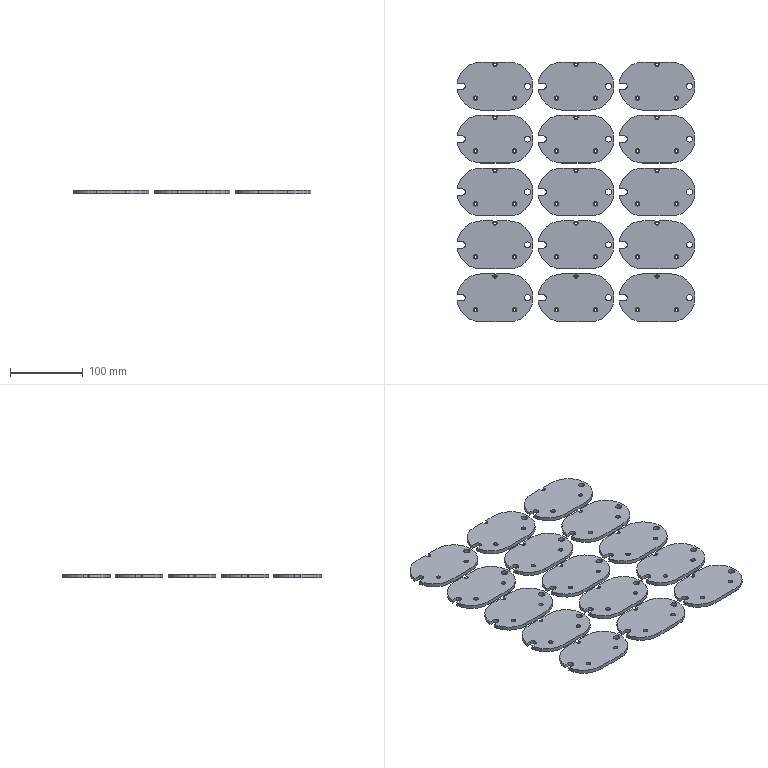NC program | NX | posted with a generic post | part box 328.125 x 358 x 5 mm
Lines 1 to 830 of 9242:
N10 G17 G21 G94 G90
(ZLEVEL_PROFILE , TOOL : D6)
N12 T06 M6
N14 G54
N16 G17 G0 G90 X177.744 Y-74.985 S7500 M3
N18 G43 Z30. H6
N20 Z1.5
N22 G94 G1 X177.771 Y-75.029 Z1.497 F1000.
N24 X179.541 Y-78.773 Z1.28
N26 X180.871 Y-82.695 Z1.063
N28 X181.745 Y-86.743 Z0.846
N30 X182.15 Y-90.864 Z0.629
N32 Y-111.837 Z-0.47
N34 Y-131.337 F2500.
N36 G2 X150.656 Y-167.186 R36.15
N38 X147.1 Y-164.035 R3.15
N40 G1 Y-156.837
N42 G3 X146. Y-155.737 R1.1
N44 X144.9 Y-156.837 R1.1
N46 G1 Y-164.063
N48 G2 X141.344 Y-167.186 R3.15
N50 X109.85 Y-131.337 R36.15
N52 G1 Y-92.337
N54 G2 X146. Y-56.187 R36.15
N56 X182.15 Y-92.337 R36.15
N58 G1 Y-111.837
N60 Y-131.284 Z-0.809
N62 X182.149 Y-131.583 Z-0.815
N64 X182.146 Y-131.883 Z-0.82
N66 X182.14 Y-132.182 Z-0.825
N68 X182.132 Y-132.481 Z-0.83
N70 X182.121 Y-132.78 Z-0.836
N72 X182.108 Y-133.079 Z-0.841
N74 X182.092 Y-133.377 Z-0.846
N76 X182.074 Y-133.676 Z-0.851
N78 X182.054 Y-133.974 Z-0.856
N80 X182.031 Y-134.273 Z-0.862
N82 X182.005 Y-134.571 Z-0.867
N84 X181.977 Y-134.869 Z-0.872
N86 X181.947 Y-135.166 Z-0.877
N88 X181.914 Y-135.464 Z-0.883
N90 X181.878 Y-135.761 Z-0.888
N92 X181.841 Y-136.058 Z-0.893
N94 X181.8 Y-136.354 Z-0.898
N96 X181.757 Y-136.65 Z-0.903
N98 X181.712 Y-136.946 Z-0.909
N100 X181.665 Y-137.241 Z-0.914
N102 X181.615 Y-137.536 Z-0.919
N104 X181.562 Y-137.831 Z-0.924
N106 X181.507 Y-138.125 Z-0.93
N108 X181.45 Y-138.418 Z-0.935
N110 X181.39 Y-138.712 Z-0.94
N112 G2 X150.656 Y-167.186 R36.15
N114 X147.1 Y-164.035 R3.15
N116 G1 Y-156.837
N118 G3 X146. Y-155.737 R1.1
N120 X144.9 Y-156.837 R1.1
N122 G1 Y-164.063
N124 G2 X141.344 Y-167.186 R3.15
N126 X109.85 Y-131.337 R36.15
N128 G1 Y-92.337
N130 G2 X146. Y-56.187 R36.15
N132 X182.15 Y-92.337 R36.15
N134 G1 Y-111.837
N136 Y-131.284 Z-1.279
N138 X182.149 Y-131.583 Z-1.285
N140 X182.146 Y-131.883 Z-1.29
N142 X182.14 Y-132.182 Z-1.295
N144 X182.132 Y-132.481 Z-1.3
N146 X182.121 Y-132.78 Z-1.306
N148 X182.108 Y-133.079 Z-1.311
N150 X182.092 Y-133.377 Z-1.316
N152 X182.074 Y-133.676 Z-1.321
N154 X182.054 Y-133.974 Z-1.326
N156 X182.031 Y-134.273 Z-1.332
N158 X182.005 Y-134.571 Z-1.337
N160 X181.977 Y-134.869 Z-1.342
N162 X181.947 Y-135.166 Z-1.347
N164 X181.914 Y-135.464 Z-1.353
N166 X181.878 Y-135.761 Z-1.358
N168 X181.841 Y-136.058 Z-1.363
N170 X181.8 Y-136.354 Z-1.368
N172 X181.757 Y-136.65 Z-1.373
N174 X181.712 Y-136.946 Z-1.379
N176 X181.665 Y-137.241 Z-1.384
N178 X181.615 Y-137.536 Z-1.389
N180 X181.562 Y-137.831 Z-1.394
N182 X181.507 Y-138.125 Z-1.4
N184 X181.45 Y-138.418 Z-1.405
N186 X181.39 Y-138.712 Z-1.41
N188 G2 X150.656 Y-167.186 R36.15
N190 X147.1 Y-164.035 R3.15
N192 G1 Y-156.837
N194 G3 X146. Y-155.737 R1.1
N196 X144.9 Y-156.837 R1.1
N198 G1 Y-164.063
N200 G2 X141.344 Y-167.186 R3.15
N202 X109.85 Y-131.337 R36.15
N204 G1 Y-92.337
N206 G2 X146. Y-56.187 R36.15
N208 X182.15 Y-92.337 R36.15
N210 G1 Y-111.837
N212 Y-131.284 Z-1.749
N214 X182.149 Y-131.583 Z-1.755
N216 X182.146 Y-131.883 Z-1.76
N218 X182.14 Y-132.182 Z-1.765
N220 X182.132 Y-132.481 Z-1.77
N222 X182.121 Y-132.78 Z-1.776
N224 X182.108 Y-133.079 Z-1.781
N226 X182.092 Y-133.377 Z-1.786
N228 X182.074 Y-133.676 Z-1.791
N230 X182.054 Y-133.974 Z-1.796
N232 X182.031 Y-134.273 Z-1.802
N234 X182.005 Y-134.571 Z-1.807
N236 X181.977 Y-134.869 Z-1.812
N238 X181.947 Y-135.166 Z-1.817
N240 X181.914 Y-135.464 Z-1.823
N242 X181.878 Y-135.761 Z-1.828
N244 X181.841 Y-136.058 Z-1.833
N246 X181.8 Y-136.354 Z-1.838
N248 X181.757 Y-136.65 Z-1.843
N250 X181.712 Y-136.946 Z-1.849
N252 X181.665 Y-137.241 Z-1.854
N254 X181.615 Y-137.536 Z-1.859
N256 X181.562 Y-137.831 Z-1.864
N258 X181.507 Y-138.125 Z-1.87
N260 X181.45 Y-138.418 Z-1.875
N262 X181.39 Y-138.712 Z-1.88
N264 G2 X150.656 Y-167.186 R36.15
N266 X147.1 Y-164.035 R3.15
N268 G1 Y-156.837
N270 G3 X146. Y-155.737 R1.1
N272 X144.9 Y-156.837 R1.1
N274 G1 Y-164.063
N276 G2 X141.344 Y-167.186 R3.15
N278 X109.85 Y-131.337 R36.15
N280 G1 Y-92.337
N282 G2 X146. Y-56.187 R36.15
N284 X182.15 Y-92.337 R36.15
N286 G1 Y-111.837
N288 Y-131.284 Z-2.219
N290 X182.149 Y-131.583 Z-2.225
N292 X182.146 Y-131.883 Z-2.23
N294 X182.14 Y-132.182 Z-2.235
N296 X182.132 Y-132.481 Z-2.24
N298 X182.121 Y-132.78 Z-2.246
N300 X182.108 Y-133.079 Z-2.251
N302 X182.092 Y-133.377 Z-2.256
N304 X182.074 Y-133.676 Z-2.261
N306 X182.054 Y-133.974 Z-2.266
N308 X182.031 Y-134.273 Z-2.272
N310 X182.005 Y-134.571 Z-2.277
N312 X181.977 Y-134.869 Z-2.282
N314 X181.947 Y-135.166 Z-2.287
N316 X181.914 Y-135.464 Z-2.293
N318 X181.878 Y-135.761 Z-2.298
N320 X181.841 Y-136.058 Z-2.303
N322 X181.8 Y-136.354 Z-2.308
N324 X181.757 Y-136.65 Z-2.313
N326 X181.712 Y-136.946 Z-2.319
N328 X181.665 Y-137.241 Z-2.324
N330 X181.615 Y-137.536 Z-2.329
N332 X181.562 Y-137.831 Z-2.334
N334 X181.507 Y-138.125 Z-2.34
N336 X181.45 Y-138.418 Z-2.345
N338 X181.39 Y-138.712 Z-2.35
N340 G2 X150.656 Y-167.186 R36.15
N342 X147.1 Y-164.035 R3.15
N344 G1 Y-156.837
N346 G3 X146. Y-155.737 R1.1
N348 X144.9 Y-156.837 R1.1
N350 G1 Y-164.063
N352 G2 X141.344 Y-167.186 R3.15
N354 X109.85 Y-131.337 R36.15
N356 G1 Y-92.337
N358 G2 X146. Y-56.187 R36.15
N360 X182.15 Y-92.337 R36.15
N362 G1 Y-111.837
N364 Y-131.284 Z-2.689
N366 X182.149 Y-131.583 Z-2.695
N368 X182.146 Y-131.883 Z-2.7
N370 X182.14 Y-132.182 Z-2.705
N372 X182.132 Y-132.481 Z-2.71
N374 X182.121 Y-132.78 Z-2.716
N376 X182.108 Y-133.079 Z-2.721
N378 X182.092 Y-133.377 Z-2.726
N380 X182.074 Y-133.676 Z-2.731
N382 X182.054 Y-133.974 Z-2.736
N384 X182.031 Y-134.273 Z-2.742
N386 X182.005 Y-134.571 Z-2.747
N388 X181.977 Y-134.869 Z-2.752
N390 X181.947 Y-135.166 Z-2.757
N392 X181.914 Y-135.464 Z-2.763
N394 X181.878 Y-135.761 Z-2.768
N396 X181.841 Y-136.058 Z-2.773
N398 X181.8 Y-136.354 Z-2.778
N400 X181.757 Y-136.65 Z-2.783
N402 X181.712 Y-136.946 Z-2.789
N404 X181.665 Y-137.241 Z-2.794
N406 X181.615 Y-137.536 Z-2.799
N408 X181.562 Y-137.831 Z-2.804
N410 X181.507 Y-138.125 Z-2.81
N412 X181.45 Y-138.418 Z-2.815
N414 X181.39 Y-138.712 Z-2.82
N416 G2 X150.656 Y-167.186 R36.15
N418 X147.1 Y-164.035 R3.15
N420 G1 Y-156.837
N422 G3 X146. Y-155.737 R1.1
N424 X144.9 Y-156.837 R1.1
N426 G1 Y-164.063
N428 G2 X141.344 Y-167.186 R3.15
N430 X109.85 Y-131.337 R36.15
N432 G1 Y-92.337
N434 G2 X146. Y-56.187 R36.15
N436 X182.15 Y-92.337 R36.15
N438 G1 Y-111.837
N440 Y-131.284 Z-3.159
N442 X182.149 Y-131.583 Z-3.165
N444 X182.146 Y-131.883 Z-3.17
N446 X182.14 Y-132.182 Z-3.175
N448 X182.132 Y-132.481 Z-3.18
N450 X182.121 Y-132.78 Z-3.186
N452 X182.108 Y-133.079 Z-3.191
N454 X182.092 Y-133.377 Z-3.196
N456 X182.074 Y-133.676 Z-3.201
N458 X182.054 Y-133.974 Z-3.206
N460 X182.031 Y-134.273 Z-3.212
N462 X182.005 Y-134.571 Z-3.217
N464 X181.977 Y-134.869 Z-3.222
N466 X181.947 Y-135.166 Z-3.227
N468 X181.914 Y-135.464 Z-3.233
N470 X181.878 Y-135.761 Z-3.238
N472 X181.841 Y-136.058 Z-3.243
N474 X181.8 Y-136.354 Z-3.248
N476 X181.757 Y-136.65 Z-3.253
N478 X181.712 Y-136.946 Z-3.259
N480 X181.665 Y-137.241 Z-3.264
N482 X181.615 Y-137.536 Z-3.269
N484 X181.562 Y-137.831 Z-3.274
N486 X181.507 Y-138.125 Z-3.28
N488 X181.45 Y-138.418 Z-3.285
N490 X181.39 Y-138.712 Z-3.29
N492 G2 X150.656 Y-167.186 R36.15
N494 X147.1 Y-164.035 R3.15
N496 G1 Y-156.837
N498 G3 X146. Y-155.737 R1.1
N500 X144.9 Y-156.837 R1.1
N502 G1 Y-164.063
N504 G2 X141.344 Y-167.186 R3.15
N506 X109.85 Y-131.337 R36.15
N508 G1 Y-92.337
N510 G2 X146. Y-56.187 R36.15
N512 X182.15 Y-92.337 R36.15
N514 G1 Y-111.837
N516 Y-131.284 Z-3.629
N518 X182.149 Y-131.583 Z-3.635
N520 X182.146 Y-131.883 Z-3.64
N522 X182.14 Y-132.182 Z-3.645
N524 X182.132 Y-132.481 Z-3.65
N526 X182.121 Y-132.78 Z-3.656
N528 X182.108 Y-133.079 Z-3.661
N530 X182.092 Y-133.377 Z-3.666
N532 X182.074 Y-133.676 Z-3.671
N534 X182.054 Y-133.974 Z-3.676
N536 X182.031 Y-134.273 Z-3.682
N538 X182.005 Y-134.571 Z-3.687
N540 X181.977 Y-134.869 Z-3.692
N542 X181.947 Y-135.166 Z-3.697
N544 X181.914 Y-135.464 Z-3.703
N546 X181.878 Y-135.761 Z-3.708
N548 X181.841 Y-136.058 Z-3.713
N550 X181.8 Y-136.354 Z-3.718
N552 X181.757 Y-136.65 Z-3.723
N554 X181.712 Y-136.946 Z-3.729
N556 X181.665 Y-137.241 Z-3.734
N558 X181.615 Y-137.536 Z-3.739
N560 X181.562 Y-137.831 Z-3.744
N562 X181.507 Y-138.125 Z-3.75
N564 X181.45 Y-138.418 Z-3.755
N566 X181.39 Y-138.712 Z-3.76
N568 G2 X150.656 Y-167.186 R36.15
N570 X147.1 Y-164.035 R3.15
N572 G1 Y-156.837
N574 G3 X146. Y-155.737 R1.1
N576 X144.9 Y-156.837 R1.1
N578 G1 Y-164.063
N580 G2 X141.344 Y-167.186 R3.15
N582 X109.85 Y-131.337 R36.15
N584 G1 Y-92.337
N586 G2 X146. Y-56.187 R36.15
N588 X182.15 Y-92.337 R36.15
N590 G1 Y-111.837
N592 Y-131.284 Z-4.099
N594 X182.149 Y-131.583 Z-4.105
N596 X182.146 Y-131.883 Z-4.11
N598 X182.14 Y-132.182 Z-4.115
N600 X182.132 Y-132.481 Z-4.12
N602 X182.121 Y-132.78 Z-4.126
N604 X182.108 Y-133.079 Z-4.131
N606 X182.092 Y-133.377 Z-4.136
N608 X182.074 Y-133.676 Z-4.141
N610 X182.054 Y-133.974 Z-4.146
N612 X182.031 Y-134.273 Z-4.152
N614 X182.005 Y-134.571 Z-4.157
N616 X181.977 Y-134.869 Z-4.162
N618 X181.947 Y-135.166 Z-4.167
N620 X181.914 Y-135.464 Z-4.173
N622 X181.878 Y-135.761 Z-4.178
N624 X181.841 Y-136.058 Z-4.183
N626 X181.8 Y-136.354 Z-4.188
N628 X181.757 Y-136.65 Z-4.193
N630 X181.712 Y-136.946 Z-4.199
N632 X181.665 Y-137.241 Z-4.204
N634 X181.615 Y-137.536 Z-4.209
N636 X181.562 Y-137.831 Z-4.214
N638 X181.507 Y-138.125 Z-4.22
N640 X181.45 Y-138.418 Z-4.225
N642 X181.39 Y-138.712 Z-4.23
N644 G2 X150.656 Y-167.186 R36.15
N646 X147.1 Y-164.035 R3.15
N648 G1 Y-156.837
N650 G3 X146. Y-155.737 R1.1
N652 X144.9 Y-156.837 R1.1
N654 G1 Y-164.063
N656 G2 X141.344 Y-167.186 R3.15
N658 X109.85 Y-131.337 R36.15
N660 G1 Y-92.337
N662 G2 X146. Y-56.187 R36.15
N664 X182.15 Y-92.337 R36.15
N666 G1 Y-111.837
N668 Y-131.284 Z-4.569
N670 X182.149 Y-131.583 Z-4.575
N672 X182.146 Y-131.883 Z-4.58
N674 X182.14 Y-132.182 Z-4.585
N676 X182.132 Y-132.481 Z-4.59
N678 X182.121 Y-132.78 Z-4.596
N680 X182.108 Y-133.079 Z-4.601
N682 X182.092 Y-133.377 Z-4.606
N684 X182.074 Y-133.676 Z-4.611
N686 X182.054 Y-133.974 Z-4.616
N688 X182.031 Y-134.273 Z-4.622
N690 X182.005 Y-134.571 Z-4.627
N692 X181.977 Y-134.869 Z-4.632
N694 X181.947 Y-135.166 Z-4.637
N696 X181.914 Y-135.464 Z-4.643
N698 X181.878 Y-135.761 Z-4.648
N700 X181.841 Y-136.058 Z-4.653
N702 X181.8 Y-136.354 Z-4.658
N704 X181.757 Y-136.65 Z-4.663
N706 X181.712 Y-136.946 Z-4.669
N708 X181.665 Y-137.241 Z-4.674
N710 X181.615 Y-137.536 Z-4.679
N712 X181.562 Y-137.831 Z-4.684
N714 X181.507 Y-138.125 Z-4.69
N716 X181.45 Y-138.418 Z-4.695
N718 X181.39 Y-138.712 Z-4.7
N720 G2 X150.656 Y-167.186 R36.15
N722 X147.1 Y-164.035 R3.15
N724 G1 Y-156.837
N726 G3 X146. Y-155.737 R1.1
N728 X144.9 Y-156.837 R1.1
N730 G1 Y-164.063
N732 G2 X141.344 Y-167.186 R3.15
N734 X109.85 Y-131.337 R36.15
N736 G1 Y-92.337
N738 G2 X146. Y-56.187 R36.15
N740 X182.15 Y-92.337 R36.15
N742 G1 Y-131.337
N744 G2 X181.39 Y-138.712 R36.15
N746 G1 Z-3.2
N748 G0 Z30.
N750 X177.744 Y36.715
N752 Z1.5
N754 G1 X177.771 Y36.671 Z1.497 F1000.
N756 X179.541 Y32.927 Z1.28
N758 X180.871 Y29.005 Z1.063
N760 X181.745 Y24.957 Z0.846
N762 X182.15 Y20.836 Z0.629
N764 Y-0.137 Z-0.47
N766 Y-19.637 F2500.
N768 G2 X150.656 Y-55.486 R36.15
N770 X147.1 Y-52.335 R3.15
N772 G1 Y-45.137
N774 G3 X146. Y-44.037 R1.1
N776 X144.9 Y-45.137 R1.1
N778 G1 Y-52.363
N780 G2 X141.344 Y-55.486 R3.15
N782 X109.85 Y-19.637 R36.15
N784 G1 Y19.363
N786 G2 X146. Y55.513 R36.15
N788 X182.15 Y19.363 R36.15
N790 G1 Y-0.137
N792 Y-19.584 Z-0.809
N794 X182.149 Y-19.883 Z-0.815
N796 X182.146 Y-20.183 Z-0.82
N798 X182.14 Y-20.482 Z-0.825
N800 X182.132 Y-20.781 Z-0.83
N802 X182.121 Y-21.08 Z-0.836
N804 X182.108 Y-21.379 Z-0.841
N806 X182.092 Y-21.677 Z-0.846
N808 X182.074 Y-21.976 Z-0.851
N810 X182.054 Y-22.274 Z-0.856
N812 X182.031 Y-22.573 Z-0.862
N814 X182.005 Y-22.871 Z-0.867
N816 X181.977 Y-23.169 Z-0.872
N818 X181.947 Y-23.466 Z-0.877
N820 X181.914 Y-23.764 Z-0.883
N822 X181.878 Y-24.061 Z-0.888
N824 X181.841 Y-24.358 Z-0.893
N826 X181.8 Y-24.654 Z-0.898
N828 X181.757 Y-24.95 Z-0.903
N830 X181.712 Y-25.246 Z-0.909
N832 X181.665 Y-25.541 Z-0.914
N834 X181.615 Y-25.836 Z-0.919
N836 X181.562 Y-26.131 Z-0.924
N838 X181.507 Y-26.425 Z-0.93
N840 X181.45 Y-26.718 Z-0.935
N842 X181.39 Y-27.012 Z-0.94
N844 G2 X150.656 Y-55.486 R36.15
N846 X147.1 Y-52.335 R3.15
N848 G1 Y-45.137
N850 G3 X146. Y-44.037 R1.1
N852 X144.9 Y-45.137 R1.1
N854 G1 Y-52.363
N856 G2 X141.344 Y-55.486 R3.15
N858 X109.85 Y-19.637 R36.15
N860 G1 Y19.363
N862 G2 X146. Y55.513 R36.15
N864 X182.15 Y19.363 R36.15
N866 G1 Y-0.137
N868 Y-19.584 Z-1.279
N870 X182.149 Y-19.883 Z-1.285
N872 X182.146 Y-20.183 Z-1.29
N874 X182.14 Y-20.482 Z-1.295
N876 X182.132 Y-20.781 Z-1.3
N878 X182.121 Y-21.08 Z-1.306
N880 X182.108 Y-21.379 Z-1.311
N882 X182.092 Y-21.677 Z-1.316
N884 X182.074 Y-21.976 Z-1.321
N886 X182.054 Y-22.274 Z-1.326
N888 X182.031 Y-22.573 Z-1.332
N890 X182.005 Y-22.871 Z-1.337
N892 X181.977 Y-23.169 Z-1.342
N894 X181.947 Y-23.466 Z-1.347
N896 X181.914 Y-23.764 Z-1.353
N898 X181.878 Y-24.061 Z-1.358
N900 X181.841 Y-24.358 Z-1.363
N902 X181.8 Y-24.654 Z-1.368
N904 X181.757 Y-24.95 Z-1.373
N906 X181.712 Y-25.246 Z-1.379
N908 X181.665 Y-25.541 Z-1.384
N910 X181.615 Y-25.836 Z-1.389
N912 X181.562 Y-26.131 Z-1.394
N914 X181.507 Y-26.425 Z-1.4
N916 X181.45 Y-26.718 Z-1.405
N918 X181.39 Y-27.012 Z-1.41
N920 G2 X150.624 Y-55.49 R36.15
N922 X147.1 Y-52.335 R3.15
N924 G1 Y-45.137
N926 G3 X146. Y-44.037 R1.1
N928 X144.9 Y-45.137 R1.1
N930 G1 Y-52.363
N932 G2 X141.344 Y-55.486 R3.15
N934 X109.85 Y-19.637 R36.15
N936 G1 Y19.363
N938 G2 X146. Y55.513 R36.15
N940 X182.15 Y19.363 R36.15
N942 G1 Y-0.137
N944 Y-19.584 Z-1.749
N946 X182.149 Y-19.883 Z-1.755
N948 X182.146 Y-20.183 Z-1.76
N950 X182.14 Y-20.482 Z-1.765
N952 X182.132 Y-20.781 Z-1.77
N954 X182.121 Y-21.08 Z-1.776
N956 X182.108 Y-21.379 Z-1.781
N958 X182.092 Y-21.677 Z-1.786
N960 X182.074 Y-21.976 Z-1.791
N962 X182.054 Y-22.274 Z-1.796
N964 X182.031 Y-22.573 Z-1.802
N966 X182.005 Y-22.871 Z-1.807
N968 X181.977 Y-23.169 Z-1.812
N970 X181.947 Y-23.466 Z-1.817
N972 X181.914 Y-23.764 Z-1.823
N974 X181.878 Y-24.061 Z-1.828
N976 X181.841 Y-24.358 Z-1.833
N978 X181.8 Y-24.654 Z-1.838
N980 X181.757 Y-24.95 Z-1.843
N982 X181.712 Y-25.246 Z-1.849
N984 X181.665 Y-25.541 Z-1.854
N986 X181.615 Y-25.836 Z-1.859
N988 X181.562 Y-26.131 Z-1.864
N990 X181.507 Y-26.425 Z-1.87
N992 X181.45 Y-26.718 Z-1.875
N994 X181.39 Y-27.012 Z-1.88
N996 G2 X150.624 Y-55.49 R36.15
N998 X147.1 Y-52.335 R3.15
N1000 G1 Y-45.137
N1002 G3 X146. Y-44.037 R1.1
N1004 X144.9 Y-45.137 R1.1
N1006 G1 Y-52.363
N1008 G2 X141.344 Y-55.486 R3.15
N1010 X109.85 Y-19.637 R36.15
N1012 G1 Y19.363
N1014 G2 X146. Y55.513 R36.15
N1016 X182.15 Y19.363 R36.15
N1018 G1 Y-0.137
N1020 Y-19.584 Z-2.219
N1022 X182.149 Y-19.883 Z-2.225
N1024 X182.146 Y-20.183 Z-2.23
N1026 X182.14 Y-20.482 Z-2.235
N1028 X182.132 Y-20.781 Z-2.24
N1030 X182.121 Y-21.08 Z-2.246
N1032 X182.108 Y-21.379 Z-2.251
N1034 X182.092 Y-21.677 Z-2.256
N1036 X182.074 Y-21.976 Z-2.261
N1038 X182.054 Y-22.274 Z-2.266
N1040 X182.031 Y-22.573 Z-2.272
N1042 X182.005 Y-22.871 Z-2.277
N1044 X181.977 Y-23.169 Z-2.282
N1046 X181.947 Y-23.466 Z-2.287
N1048 X181.914 Y-23.764 Z-2.293
N1050 X181.878 Y-24.061 Z-2.298
N1052 X181.841 Y-24.358 Z-2.303
N1054 X181.8 Y-24.654 Z-2.308
N1056 X181.757 Y-24.95 Z-2.313
N1058 X181.712 Y-25.246 Z-2.319
N1060 X181.665 Y-25.541 Z-2.324
N1062 X181.615 Y-25.836 Z-2.329
N1064 X181.562 Y-26.131 Z-2.334
N1066 X181.507 Y-26.425 Z-2.34
N1068 X181.45 Y-26.718 Z-2.345
N1070 X181.39 Y-27.012 Z-2.35
N1072 G2 X150.624 Y-55.49 R36.15
N1074 X147.1 Y-52.335 R3.15
N1076 G1 Y-45.137
N1078 G3 X146. Y-44.037 R1.1
N1080 X144.9 Y-45.137 R1.1
N1082 G1 Y-52.363
N1084 G2 X141.344 Y-55.486 R3.15
N1086 X109.85 Y-19.637 R36.15
N1088 G1 Y19.363
N1090 G2 X146. Y55.513 R36.15
N1092 X182.15 Y19.363 R36.15
N1094 G1 Y-0.137
N1096 Y-19.584 Z-2.689
N1098 X182.149 Y-19.883 Z-2.695
N1100 X182.146 Y-20.183 Z-2.7
N1102 X182.14 Y-20.482 Z-2.705
N1104 X182.132 Y-20.781 Z-2.71
N1106 X182.121 Y-21.08 Z-2.716
N1108 X182.108 Y-21.379 Z-2.721
N1110 X182.092 Y-21.677 Z-2.726
N1112 X182.074 Y-21.976 Z-2.731
N1114 X182.054 Y-22.274 Z-2.736
N1116 X182.031 Y-22.573 Z-2.742
N1118 X182.005 Y-22.871 Z-2.747
N1120 X181.977 Y-23.169 Z-2.752
N1122 X181.947 Y-23.466 Z-2.757
N1124 X181.914 Y-23.764 Z-2.763
N1126 X181.878 Y-24.061 Z-2.768
N1128 X181.841 Y-24.358 Z-2.773
N1130 X181.8 Y-24.654 Z-2.778
N1132 X181.757 Y-24.95 Z-2.783
N1134 X181.712 Y-25.246 Z-2.789
N1136 X181.665 Y-25.541 Z-2.794
N1138 X181.615 Y-25.836 Z-2.799
N1140 X181.562 Y-26.131 Z-2.804
N1142 X181.507 Y-26.425 Z-2.81
N1144 X181.45 Y-26.718 Z-2.815
N1146 X181.39 Y-27.012 Z-2.82
N1148 G2 X150.624 Y-55.49 R36.15
N1150 X147.1 Y-52.335 R3.15
N1152 G1 Y-45.137
N1154 G3 X146. Y-44.037 R1.1
N1156 X144.9 Y-45.137 R1.1
N1158 G1 Y-52.363
N1160 G2 X141.344 Y-55.486 R3.15
N1162 X109.85 Y-19.637 R36.15
N1164 G1 Y19.363
N1166 G2 X146. Y55.513 R36.15
N1168 X182.15 Y19.363 R36.15
N1170 G1 Y-0.137
N1172 Y-19.584 Z-3.159
N1174 X182.149 Y-19.883 Z-3.165
N1176 X182.146 Y-20.183 Z-3.17
N1178 X182.14 Y-20.482 Z-3.175
N1180 X182.132 Y-20.781 Z-3.18
N1182 X182.121 Y-21.08 Z-3.186
N1184 X182.108 Y-21.379 Z-3.191
N1186 X182.092 Y-21.677 Z-3.196
N1188 X182.074 Y-21.976 Z-3.201
N1190 X182.054 Y-22.274 Z-3.206
N1192 X182.031 Y-22.573 Z-3.212
N1194 X182.005 Y-22.871 Z-3.217
N1196 X181.977 Y-23.169 Z-3.222
N1198 X181.947 Y-23.466 Z-3.227
N1200 X181.914 Y-23.764 Z-3.233
N1202 X181.878 Y-24.061 Z-3.238
N1204 X181.841 Y-24.358 Z-3.243
N1206 X181.8 Y-24.654 Z-3.248
N1208 X181.757 Y-24.95 Z-3.253
N1210 X181.712 Y-25.246 Z-3.259
N1212 X181.665 Y-25.541 Z-3.264
N1214 X181.615 Y-25.836 Z-3.269
N1216 X181.562 Y-26.131 Z-3.274
N1218 X181.507 Y-26.425 Z-3.28
N1220 X181.45 Y-26.718 Z-3.285
N1222 X181.39 Y-27.012 Z-3.29
N1224 G2 X150.624 Y-55.49 R36.15
N1226 X147.1 Y-52.335 R3.15
N1228 G1 Y-45.137
N1230 G3 X146. Y-44.037 R1.1
N1232 X144.9 Y-45.137 R1.1
N1234 G1 Y-52.363
N1236 G2 X141.344 Y-55.486 R3.15
N1238 X109.85 Y-19.637 R36.15
N1240 G1 Y19.363
N1242 G2 X146. Y55.513 R36.15
N1244 X182.15 Y19.363 R36.15
N1246 G1 Y-0.137
N1248 Y-19.584 Z-3.629
N1250 X182.149 Y-19.883 Z-3.635
N1252 X182.146 Y-20.183 Z-3.64
N1254 X182.14 Y-20.482 Z-3.645
N1256 X182.132 Y-20.781 Z-3.65
N1258 X182.121 Y-21.08 Z-3.656
N1260 X182.108 Y-21.379 Z-3.661
N1262 X182.092 Y-21.677 Z-3.666
N1264 X182.074 Y-21.976 Z-3.671
N1266 X182.054 Y-22.274 Z-3.676
N1268 X182.031 Y-22.573 Z-3.682
N1270 X182.005 Y-22.871 Z-3.687
N1272 X181.977 Y-23.169 Z-3.692
N1274 X181.947 Y-23.466 Z-3.697
N1276 X181.914 Y-23.764 Z-3.703
N1278 X181.878 Y-24.061 Z-3.708
N1280 X181.841 Y-24.358 Z-3.713
N1282 X181.8 Y-24.654 Z-3.718
N1284 X181.757 Y-24.95 Z-3.723
N1286 X181.712 Y-25.246 Z-3.729
N1288 X181.665 Y-25.541 Z-3.734
N1290 X181.615 Y-25.836 Z-3.739
N1292 X181.562 Y-26.131 Z-3.744
N1294 X181.507 Y-26.425 Z-3.75
N1296 X181.45 Y-26.718 Z-3.755
N1298 X181.39 Y-27.012 Z-3.76
N1300 G2 X150.624 Y-55.49 R36.15
N1302 X147.1 Y-52.335 R3.15
N1304 G1 Y-45.137
N1306 G3 X146. Y-44.037 R1.1
N1308 X144.9 Y-45.137 R1.1
N1310 G1 Y-52.363
N1312 G2 X141.344 Y-55.486 R3.15
N1314 X109.85 Y-19.637 R36.15
N1316 G1 Y19.363
N1318 G2 X146. Y55.513 R36.15
N1320 X182.15 Y19.363 R36.15
N1322 G1 Y-0.137
N1324 Y-19.584 Z-4.099
N1326 X182.149 Y-19.883 Z-4.105
N1328 X182.146 Y-20.183 Z-4.11
N1330 X182.14 Y-20.482 Z-4.115
N1332 X182.132 Y-20.781 Z-4.12
N1334 X182.121 Y-21.08 Z-4.126
N1336 X182.108 Y-21.379 Z-4.131
N1338 X182.092 Y-21.677 Z-4.136
N1340 X182.074 Y-21.976 Z-4.141
N1342 X182.054 Y-22.274 Z-4.146
N1344 X182.031 Y-22.573 Z-4.152
N1346 X182.005 Y-22.871 Z-4.157
N1348 X181.977 Y-23.169 Z-4.162
N1350 X181.947 Y-23.466 Z-4.167
N1352 X181.914 Y-23.764 Z-4.173
N1354 X181.878 Y-24.061 Z-4.178
N1356 X181.841 Y-24.358 Z-4.183
N1358 X181.8 Y-24.654 Z-4.188
N1360 X181.757 Y-24.95 Z-4.193
N1362 X181.712 Y-25.246 Z-4.199
N1364 X181.665 Y-25.541 Z-4.204
N1366 X181.615 Y-25.836 Z-4.209
N1368 X181.562 Y-26.131 Z-4.214
N1370 X181.507 Y-26.425 Z-4.22
N1372 X181.45 Y-26.718 Z-4.225
N1374 X181.39 Y-27.012 Z-4.23
N1376 G2 X150.624 Y-55.49 R36.15
N1378 X147.1 Y-52.335 R3.15
N1380 G1 Y-45.137
N1382 G3 X146. Y-44.037 R1.1
N1384 X144.9 Y-45.137 R1.1
N1386 G1 Y-52.363
N1388 G2 X141.344 Y-55.486 R3.15
N1390 X109.85 Y-19.637 R36.15
N1392 G1 Y19.363
N1394 G2 X146. Y55.513 R36.15
N1396 X182.15 Y19.363 R36.15
N1398 G1 Y-0.137
N1400 Y-19.584 Z-4.569
N1402 X182.149 Y-19.883 Z-4.575
N1404 X182.146 Y-20.183 Z-4.58
N1406 X182.14 Y-20.482 Z-4.585
N1408 X182.132 Y-20.781 Z-4.59
N1410 X182.121 Y-21.08 Z-4.596
N1412 X182.108 Y-21.379 Z-4.601
N1414 X182.092 Y-21.677 Z-4.606
N1416 X182.074 Y-21.976 Z-4.611
N1418 X182.054 Y-22.274 Z-4.616
N1420 X182.031 Y-22.573 Z-4.622
N1422 X182.005 Y-22.871 Z-4.627
N1424 X181.977 Y-23.169 Z-4.632
N1426 X181.947 Y-23.466 Z-4.637
N1428 X181.914 Y-23.764 Z-4.643
N1430 X181.878 Y-24.061 Z-4.648
N1432 X181.841 Y-24.358 Z-4.653
N1434 X181.8 Y-24.654 Z-4.658
N1436 X181.757 Y-24.95 Z-4.663
N1438 X181.712 Y-25.246 Z-4.669
N1440 X181.665 Y-25.541 Z-4.674
N1442 X181.615 Y-25.836 Z-4.679
N1444 X181.562 Y-26.131 Z-4.684
N1446 X181.507 Y-26.425 Z-4.69
N1448 X181.45 Y-26.718 Z-4.695
N1450 X181.39 Y-27.012 Z-4.7
N1452 G2 X150.624 Y-55.49 R36.15
N1454 X147.1 Y-52.335 R3.15
N1456 G1 Y-45.137
N1458 G3 X146. Y-44.037 R1.1
N1460 X144.9 Y-45.137 R1.1
N1462 G1 Y-52.363
N1464 G2 X141.344 Y-55.486 R3.15
N1466 X109.85 Y-19.637 R36.15
N1468 G1 Y19.363
N1470 G2 X146. Y55.513 R36.15
N1472 X182.15 Y19.363 R36.15
N1474 G1 Y-19.637
N1476 G2 X181.39 Y-27.012 R36.15
N1478 G1 Z-3.2
N1480 G0 Z30.
N1482 X177.744 Y148.415
N1484 Z1.5
N1486 G1 X177.771 Y148.371 Z1.497 F1000.
N1488 X179.541 Y144.627 Z1.28
N1490 X180.871 Y140.705 Z1.063
N1492 X181.745 Y136.657 Z0.846
N1494 X182.15 Y132.536 Z0.629
N1496 Y111.563 Z-0.47
N1498 Y92.063 F2500.
N1500 G2 X150.656 Y56.214 R36.15
N1502 X147.1 Y59.337 R3.15
N1504 G1 Y66.563
N1506 G3 X146. Y67.663 R1.1
N1508 X144.9 Y66.563 R1.1
N1510 G1 Y59.337
N1512 G2 X141.344 Y56.214 R3.15
N1514 X109.85 Y92.063 R36.15
N1516 G1 Y131.063
N1518 G2 X146. Y167.213 R36.15
N1520 X182.15 Y131.063 R36.15
N1522 G1 Y111.563
N1524 Y92.116 Z-0.809
N1526 X182.149 Y91.817 Z-0.815
N1528 X182.146 Y91.517 Z-0.82
N1530 X182.14 Y91.218 Z-0.825
N1532 X182.132 Y90.919 Z-0.83
N1534 X182.121 Y90.62 Z-0.836
N1536 X182.108 Y90.321 Z-0.841
N1538 X182.092 Y90.023 Z-0.846
N1540 X182.074 Y89.724 Z-0.851
N1542 X182.054 Y89.426 Z-0.856
N1544 X182.031 Y89.127 Z-0.862
N1546 X182.005 Y88.829 Z-0.867
N1548 X181.977 Y88.531 Z-0.872
N1550 X181.947 Y88.234 Z-0.877
N1552 X181.914 Y87.936 Z-0.883
N1554 X181.878 Y87.639 Z-0.888
N1556 X181.841 Y87.342 Z-0.893
N1558 X181.8 Y87.046 Z-0.898
N1560 X181.757 Y86.75 Z-0.903
N1562 X181.712 Y86.454 Z-0.909
N1564 X181.665 Y86.159 Z-0.914
N1566 X181.615 Y85.864 Z-0.919
N1568 X181.562 Y85.569 Z-0.924
N1570 X181.507 Y85.275 Z-0.93
N1572 X181.45 Y84.982 Z-0.935
N1574 X181.39 Y84.688 Z-0.94
N1576 G2 X150.656 Y56.214 R36.15
N1578 X147.1 Y59.337 R3.15
N1580 G1 Y66.563
N1582 G3 X146. Y67.663 R1.1
N1584 X144.9 Y66.563 R1.1
N1586 G1 Y59.337
N1588 G2 X141.344 Y56.214 R3.15
N1590 X109.85 Y92.063 R36.15
N1592 G1 Y131.063
N1594 G2 X146. Y167.213 R36.15
N1596 X182.15 Y131.063 R36.15
N1598 G1 Y111.563
N1600 Y92.116 Z-1.279
N1602 X182.149 Y91.817 Z-1.285
N1604 X182.146 Y91.517 Z-1.29
N1606 X182.14 Y91.218 Z-1.295
N1608 X182.132 Y90.919 Z-1.3
N1610 X182.121 Y90.62 Z-1.306
N1612 X182.108 Y90.321 Z-1.311
N1614 X182.092 Y90.023 Z-1.316
N1616 X182.074 Y89.724 Z-1.321
N1618 X182.054 Y89.426 Z-1.326
N1620 X182.031 Y89.127 Z-1.332
N1622 X182.005 Y88.829 Z-1.337
N1624 X181.977 Y88.531 Z-1.342
N1626 X181.947 Y88.234 Z-1.347
N1628 X181.914 Y87.936 Z-1.353
N1630 X181.878 Y87.639 Z-1.358
N1632 X181.841 Y87.342 Z-1.363
N1634 X181.8 Y87.046 Z-1.368
N1636 X181.757 Y86.75 Z-1.373
N1638 X181.712 Y86.454 Z-1.379
N1640 X181.665 Y86.159 Z-1.384
N1642 X181.615 Y85.864 Z-1.389
N1644 X181.562 Y85.569 Z-1.394
N1646 X181.507 Y85.275 Z-1.4
N1648 X181.45 Y84.982 Z-1.405
N1650 X181.39 Y84.688 Z-1.41
N1652 G2 X150.656 Y56.214 R36.15
N1654 X147.1 Y59.337 R3.15
N1656 G1 Y66.563
N1658 G3 X146. Y67.663 R1.1